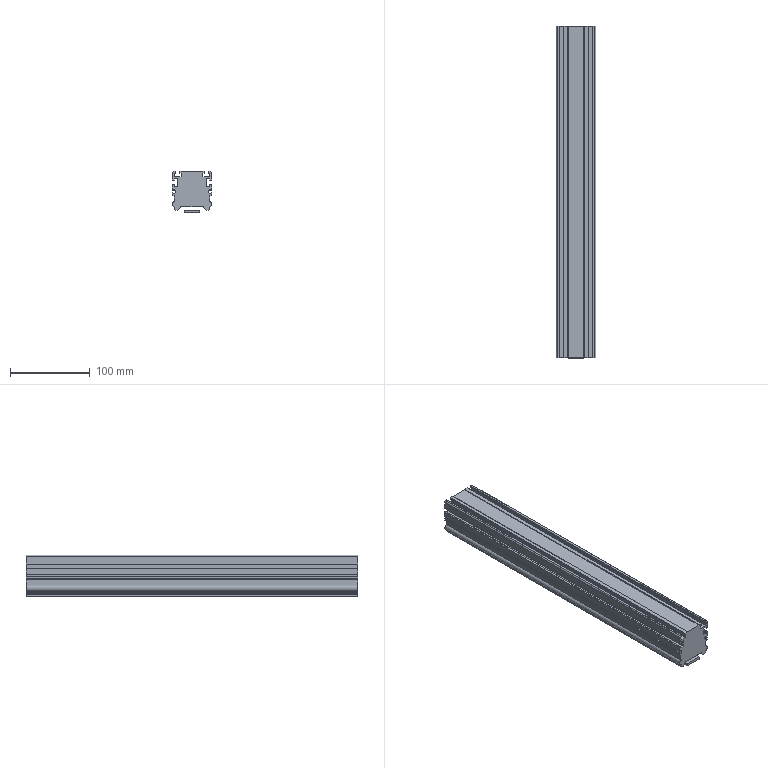Part | STEP file | Copy of 50-2016 profile^K50A-1H20-S(equation-driven)-L0 | 2 solids | 143 faces | box 50 x 415 x 52.45 mm | volume 841262 mm3 | plane 72 | cylinder 71 | commonest cylinder face diameters 0.4 x58 4.2 x6 4 x5 8 x2